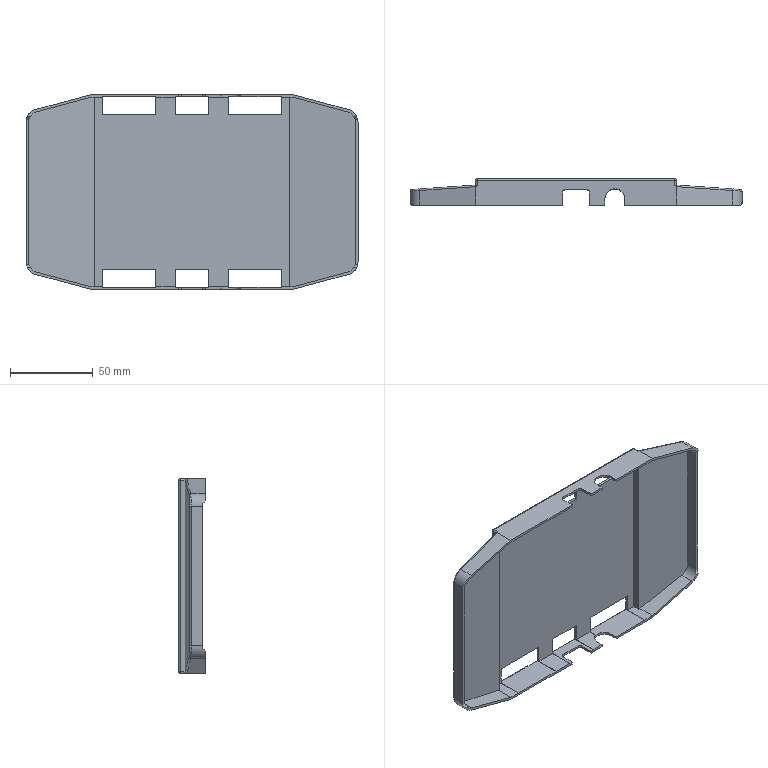Part | STEP file | LES120 top cover^FTH120-PD-direct-drive motor | 1 solid | 114 faces | box 201 x 16.2 x 118 mm | volume 41250 mm3 | plane 78 | cylinder 28 | spline 8 | commonest cylinder face diameters 2 x14 3 x4 13 x4 16 x4 12 x2